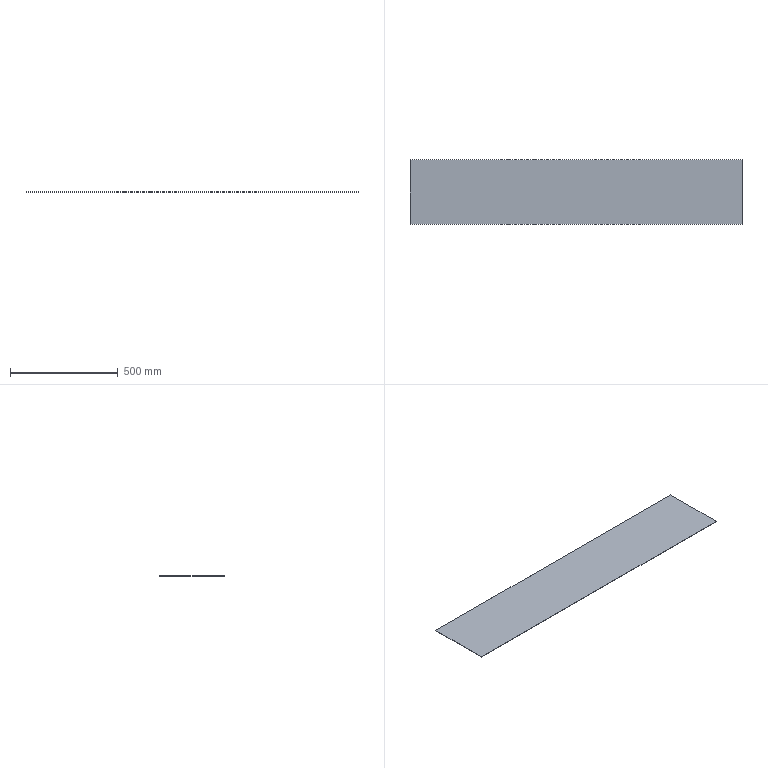Part | STEP file | X77-03026 | 1 solid | 6 faces | box 1540 x 300 x 1.5 mm | volume 693000 mm3 | plane 6
STEP:
#1=CARTESIAN_POINT('',(-682.443,-934.766,0.));
#2=VERTEX_POINT('',#1);
#3=CARTESIAN_POINT('',(-682.443,-1234.766,0.));
#4=VERTEX_POINT('',#3);
#5=CARTESIAN_POINT('',(-682.443,-934.766,0.));
#6=DIRECTION('',(0.,-1.,0.));
#7=VECTOR('',#6,1000.);
#8=LINE('',#5,#7);
#9=EDGE_CURVE('',#2,#4,#8,.T.);
#10=ORIENTED_EDGE('',*,*,#9,.F.);
#11=CARTESIAN_POINT('',(-682.443,-934.766,-1.5));
#12=VERTEX_POINT('',#11);
#13=CARTESIAN_POINT('',(-682.443,-934.766,-1.5));
#14=DIRECTION('',(0.,0.,1.));
#15=VECTOR('',#14,1000.);
#16=LINE('',#13,#15);
#17=EDGE_CURVE('',#12,#2,#16,.T.);
#18=ORIENTED_EDGE('',*,*,#17,.F.);
#19=CARTESIAN_POINT('',(-682.443,-1234.766,-1.5));
#20=VERTEX_POINT('',#19);
#21=CARTESIAN_POINT('',(-682.443,-934.766,-1.5));
#22=DIRECTION('',(0.,-1.,0.));
#23=VECTOR('',#22,1000.);
#24=LINE('',#21,#23);
#25=EDGE_CURVE('',#12,#20,#24,.T.);
#26=ORIENTED_EDGE('',*,*,#25,.T.);
#27=CARTESIAN_POINT('',(-682.443,-1234.766,-1.5));
#28=DIRECTION('',(0.,0.,1.));
#29=VECTOR('',#28,1000.);
#30=LINE('',#27,#29);
#31=EDGE_CURVE('',#20,#4,#30,.T.);
#32=ORIENTED_EDGE('',*,*,#31,.T.);
#33=EDGE_LOOP('',(#10,#18,#26,#32));
#34=FACE_OUTER_BOUND('',#33,.T.);
#35=CARTESIAN_POINT('',(-682.443,-934.766,-1.5));
#36=DIRECTION('',(-1.,0.,0.));
#37=DIRECTION('',(0.,0.,1.));
#38=AXIS2_PLACEMENT_3D('',#35,#36,#37);
#39=PLANE('',#38);
#40=ADVANCED_FACE('',(#34),#39,.T.);
#41=CARTESIAN_POINT('',(857.557,-934.766,0.));
#42=VERTEX_POINT('',#41);
#43=CARTESIAN_POINT('',(-682.443,-934.766,0.));
#44=DIRECTION('',(-1.,0.,0.));
#45=VECTOR('',#44,1000.);
#46=LINE('',#43,#45);
#47=EDGE_CURVE('',#42,#2,#46,.T.);
#48=ORIENTED_EDGE('',*,*,#47,.F.);
#49=CARTESIAN_POINT('',(857.557,-934.766,-1.5));
#50=VERTEX_POINT('',#49);
#51=CARTESIAN_POINT('',(857.557,-934.766,-1.5));
#52=DIRECTION('',(0.,0.,1.));
#53=VECTOR('',#52,1000.);
#54=LINE('',#51,#53);
#55=EDGE_CURVE('',#50,#42,#54,.T.);
#56=ORIENTED_EDGE('',*,*,#55,.F.);
#57=CARTESIAN_POINT('',(-682.443,-934.766,-1.5));
#58=DIRECTION('',(-1.,0.,0.));
#59=VECTOR('',#58,1000.);
#60=LINE('',#57,#59);
#61=EDGE_CURVE('',#50,#12,#60,.T.);
#62=ORIENTED_EDGE('',*,*,#61,.T.);
#63=ORIENTED_EDGE('',*,*,#17,.T.);
#64=EDGE_LOOP('',(#48,#56,#62,#63));
#65=FACE_OUTER_BOUND('',#64,.T.);
#66=CARTESIAN_POINT('',(-682.443,-934.766,-1.5));
#67=DIRECTION('',(0.,1.,0.));
#68=DIRECTION('',(0.,0.,1.));
#69=AXIS2_PLACEMENT_3D('',#66,#67,#68);
#70=PLANE('',#69);
#71=ADVANCED_FACE('',(#65),#70,.T.);
#72=CARTESIAN_POINT('',(857.557,-1234.766,0.));
#73=VERTEX_POINT('',#72);
#74=CARTESIAN_POINT('',(857.557,-934.766,0.));
#75=DIRECTION('',(0.,1.,0.));
#76=VECTOR('',#75,1000.);
#77=LINE('',#74,#76);
#78=EDGE_CURVE('',#73,#42,#77,.T.);
#79=ORIENTED_EDGE('',*,*,#78,.F.);
#80=CARTESIAN_POINT('',(857.557,-1234.766,-1.5));
#81=VERTEX_POINT('',#80);
#82=CARTESIAN_POINT('',(857.557,-1234.766,-1.5));
#83=DIRECTION('',(0.,0.,1.));
#84=VECTOR('',#83,1000.);
#85=LINE('',#82,#84);
#86=EDGE_CURVE('',#81,#73,#85,.T.);
#87=ORIENTED_EDGE('',*,*,#86,.F.);
#88=CARTESIAN_POINT('',(857.557,-934.766,-1.5));
#89=DIRECTION('',(0.,1.,0.));
#90=VECTOR('',#89,1000.);
#91=LINE('',#88,#90);
#92=EDGE_CURVE('',#81,#50,#91,.T.);
#93=ORIENTED_EDGE('',*,*,#92,.T.);
#94=ORIENTED_EDGE('',*,*,#55,.T.);
#95=EDGE_LOOP('',(#79,#87,#93,#94));
#96=FACE_OUTER_BOUND('',#95,.T.);
#97=CARTESIAN_POINT('',(857.557,-934.766,-1.5));
#98=DIRECTION('',(1.,0.,0.));
#99=DIRECTION('',(0.,1.,0.));
#100=AXIS2_PLACEMENT_3D('',#97,#98,#99);
#101=PLANE('',#100);
#102=ADVANCED_FACE('',(#96),#101,.T.);
#103=CARTESIAN_POINT('',(-682.443,-1234.766,0.));
#104=DIRECTION('',(1.,0.,0.));
#105=VECTOR('',#104,1000.);
#106=LINE('',#103,#105);
#107=EDGE_CURVE('',#4,#73,#106,.T.);
#108=ORIENTED_EDGE('',*,*,#107,.F.);
#109=ORIENTED_EDGE('',*,*,#31,.F.);
#110=CARTESIAN_POINT('',(-682.443,-1234.766,-1.5));
#111=DIRECTION('',(1.,0.,0.));
#112=VECTOR('',#111,1000.);
#113=LINE('',#110,#112);
#114=EDGE_CURVE('',#20,#81,#113,.T.);
#115=ORIENTED_EDGE('',*,*,#114,.T.);
#116=ORIENTED_EDGE('',*,*,#86,.T.);
#117=EDGE_LOOP('',(#108,#109,#115,#116));
#118=FACE_OUTER_BOUND('',#117,.T.);
#119=CARTESIAN_POINT('',(-682.443,-1234.766,-1.5));
#120=DIRECTION('',(0.,-1.,0.));
#121=DIRECTION('',(0.,0.,-1.));
#122=AXIS2_PLACEMENT_3D('',#119,#120,#121);
#123=PLANE('',#122);
#124=ADVANCED_FACE('',(#118),#123,.T.);
#125=ORIENTED_EDGE('',*,*,#25,.F.);
#126=ORIENTED_EDGE('',*,*,#61,.F.);
#127=ORIENTED_EDGE('',*,*,#92,.F.);
#128=ORIENTED_EDGE('',*,*,#114,.F.);
#129=EDGE_LOOP('',(#125,#126,#127,#128));
#130=FACE_OUTER_BOUND('',#129,.T.);
#131=CARTESIAN_POINT('',(-682.443,-1234.766,-1.5));
#132=DIRECTION('',(0.,0.,1.));
#133=DIRECTION('',(1.,0.,0.));
#134=AXIS2_PLACEMENT_3D('',#131,#132,#133);
#135=PLANE('',#134);
#136=ADVANCED_FACE('',(#130),#135,.F.);
#137=ORIENTED_EDGE('',*,*,#9,.T.);
#138=ORIENTED_EDGE('',*,*,#107,.T.);
#139=ORIENTED_EDGE('',*,*,#78,.T.);
#140=ORIENTED_EDGE('',*,*,#47,.T.);
#141=EDGE_LOOP('',(#137,#138,#139,#140));
#142=FACE_OUTER_BOUND('',#141,.T.);
#143=CARTESIAN_POINT('',(-682.443,-1234.766,0.));
#144=DIRECTION('',(0.,0.,1.));
#145=DIRECTION('',(1.,0.,0.));
#146=AXIS2_PLACEMENT_3D('',#143,#144,#145);
#147=PLANE('',#146);
#148=ADVANCED_FACE('',(#142),#147,.T.);
#149=CLOSED_SHELL('',(#40,#71,#102,#124,#136,#148));
#150=MANIFOLD_SOLID_BREP('',#149);
#151=CARTESIAN_POINT('',(0.,0.,0.));
#152=DIRECTION('',(0.,0.,1.));
#153=DIRECTION('',(1.,0.,0.));
#154=AXIS2_PLACEMENT_3D('',#151,#152,#153);
#155=(LENGTH_UNIT()NAMED_UNIT(*)SI_UNIT(.MILLI.,.METRE.));
#156=UNCERTAINTY_MEASURE_WITH_UNIT(LENGTH_MEASURE(0.00001),#155,'','');
#157=(NAMED_UNIT(*)PLANE_ANGLE_UNIT()SI_UNIT($,.RADIAN.));
#158=(NAMED_UNIT(*)SI_UNIT($,.STERADIAN.)SOLID_ANGLE_UNIT());
#159=(GEOMETRIC_REPRESENTATION_CONTEXT(3)GLOBAL_UNCERTAINTY_ASSIGNED_CONTEXT((#156))GLOBAL_UNIT_ASSIGNED_CONTEXT((#155,#157,#158))REPRESENTATION_CONTEXT('',''));
#160=ADVANCED_BREP_SHAPE_REPRESENTATION('',(#150,#154),#159);